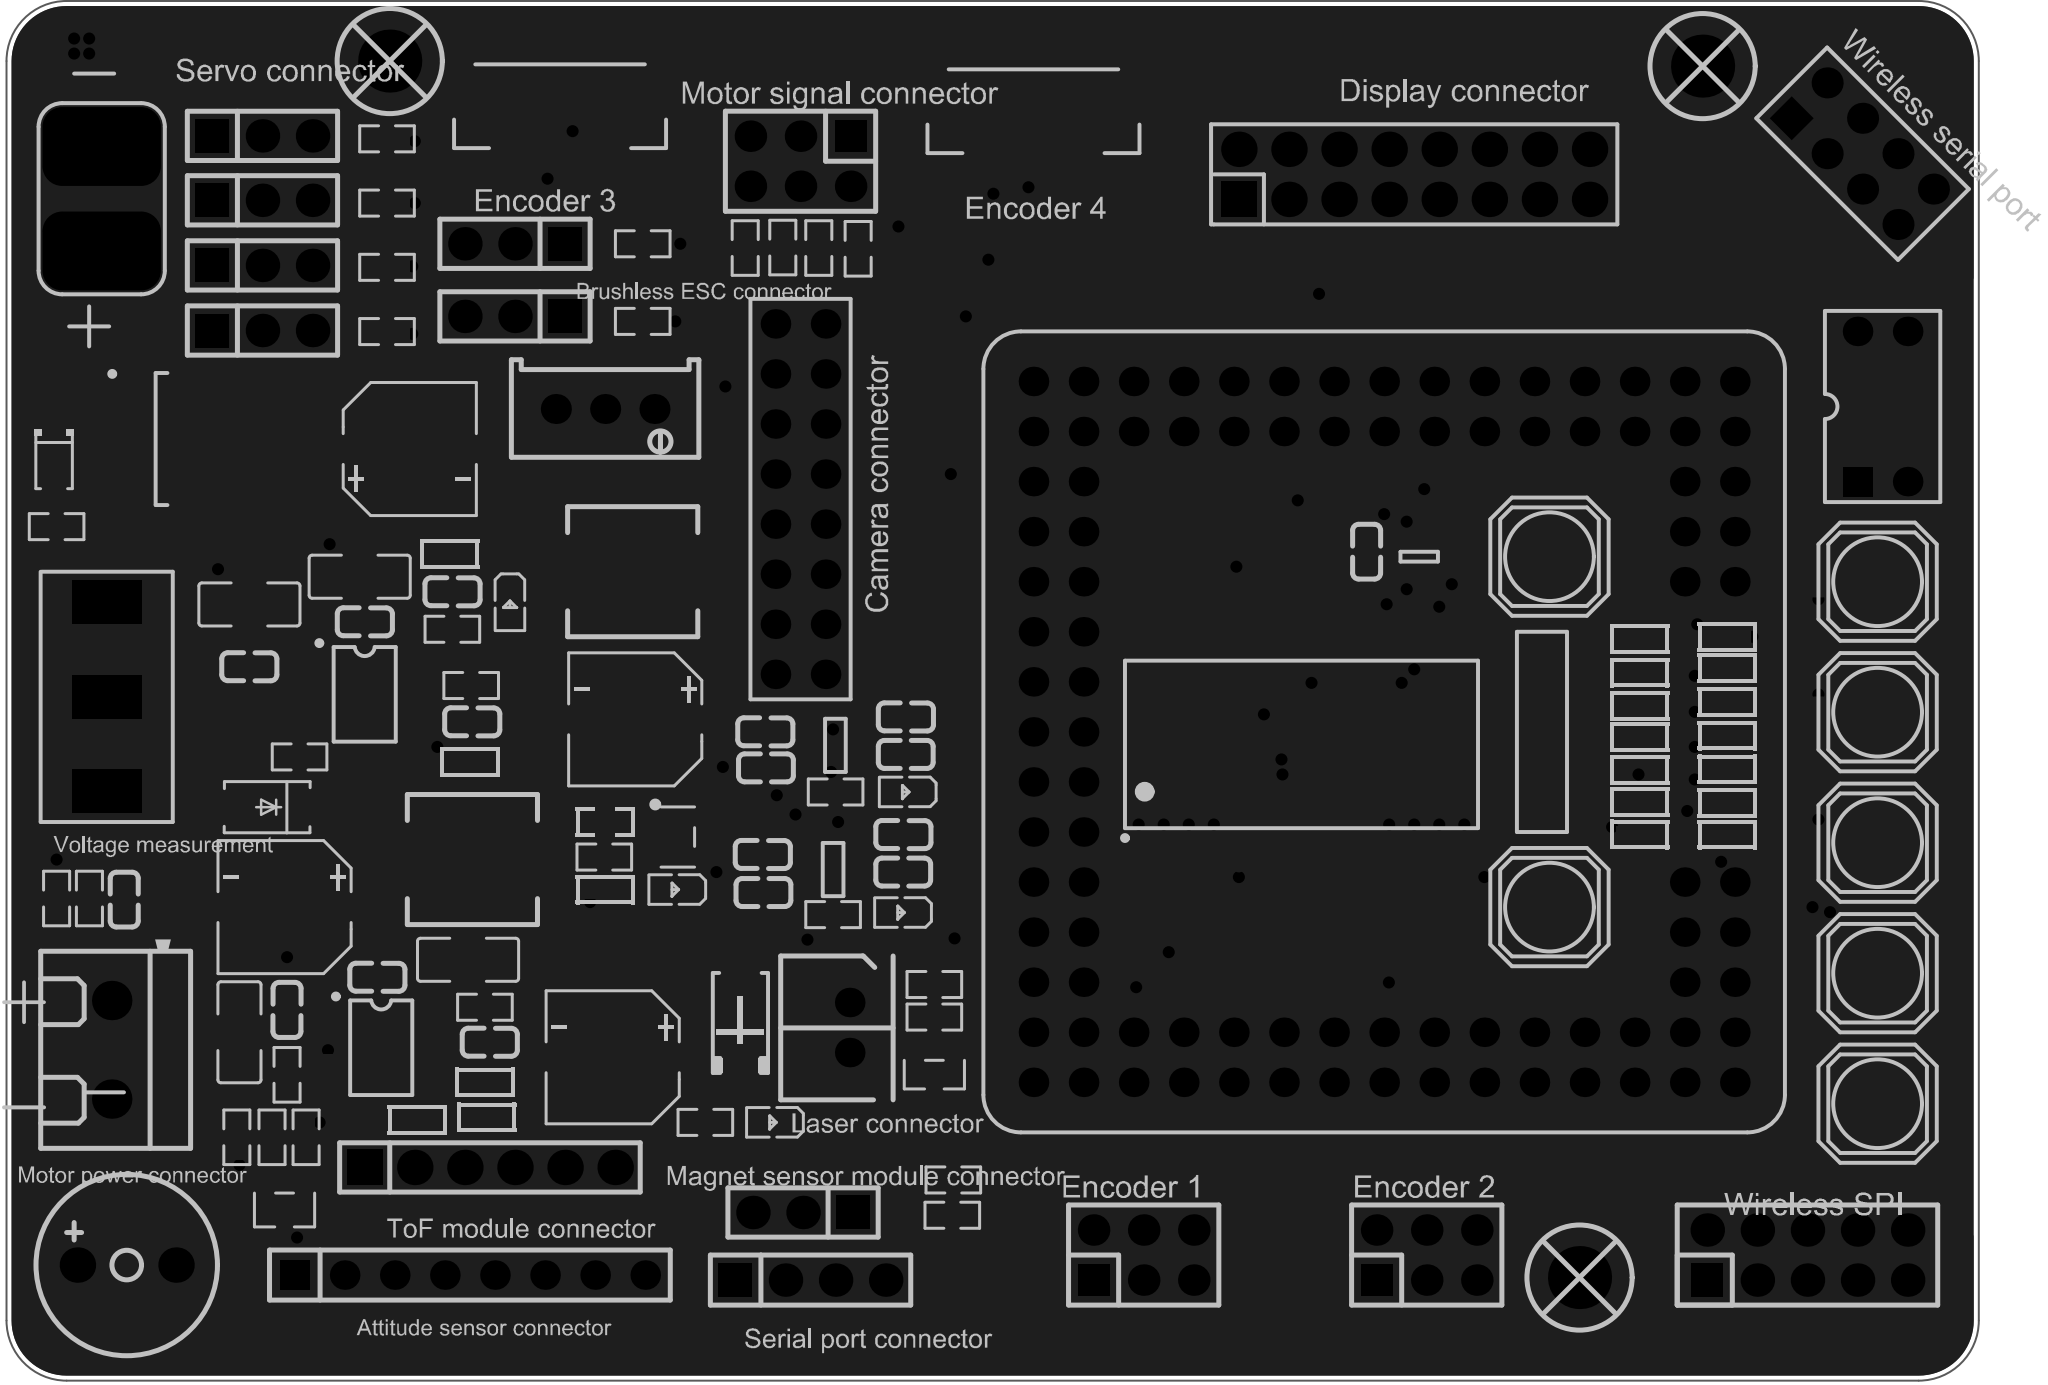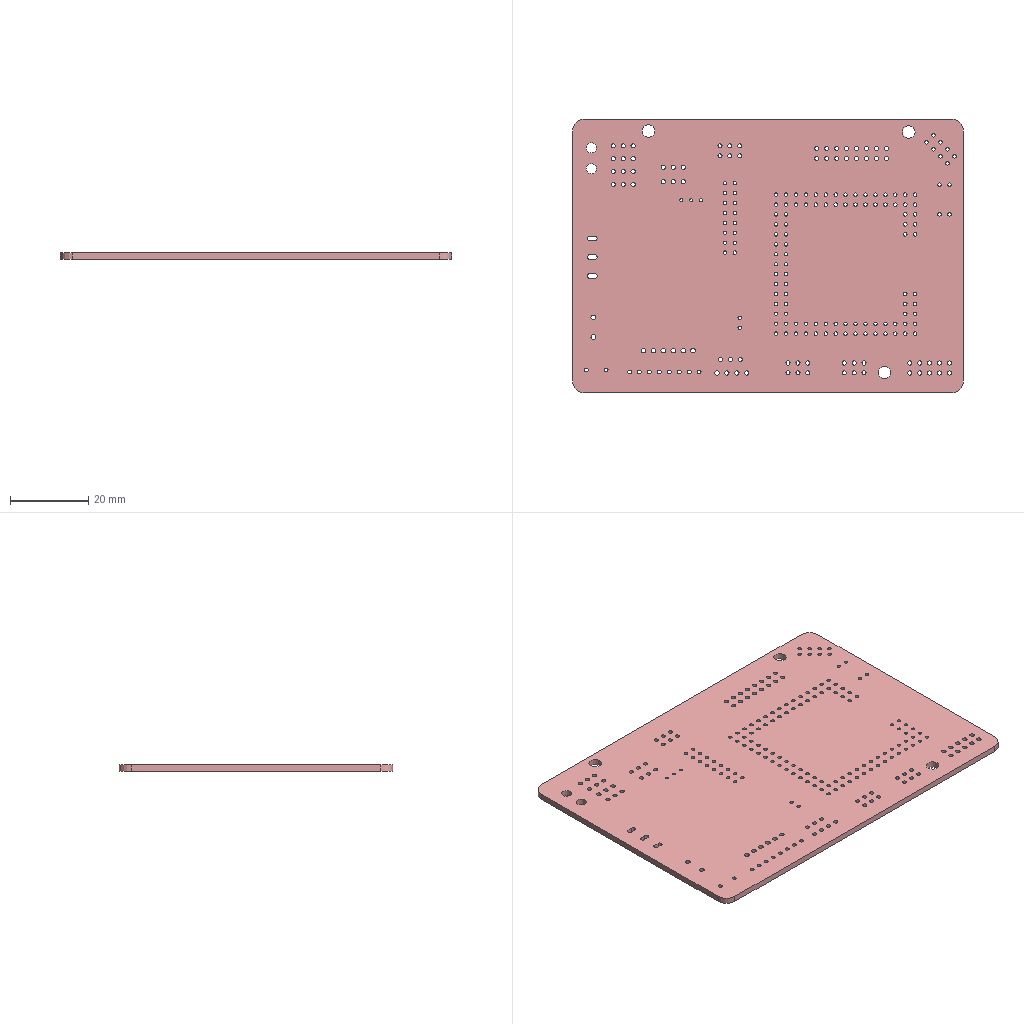Circuit board layout | Altium Designer | box 100 x 70 x 1.6 mm
Layer stack:
# Altium Designer layer stack of  (unit mm; dielectric type: 0 none, 1 core, 2 prepreg, 3 surface material)
index,name,kind,layer,copper_thickness_mm,dielectric_type,dielectric_thickness_mm,dielectric_material,dielectric_constant
0,Top Paste Mask Layer,other,,,,,,
1,Top Silkscreen Layer,other,,,,,,
2,Top Solder Mask Layer,dielectric,,,3,0,,0
3,Top Layer,copper,Top Layer,0.035,,,,
4,Dielectric1,dielectric,,,3,0.2104,7628 RC49% 8.6mil,0
5,Inner1,copper,Inner1,0.0152,,,,
6,Dielectric2,dielectric,,,3,1.065,1.1mm H/HOZ Copper,0
7,Inner2,copper,Inner2,0.0152,,,,
8,Dielectric3,dielectric,,,3,0.2104,7628 RC49% 8.6mil,0
9,Bottom Layer,copper,Bottom Layer,0.035,,,,
10,Bottom Solder Mask Layer,dielectric,,,3,0,,0
11,Bottom Silkscreen Layer,other,,,,,,
12,Bottom Paste Mask Layer,other,,,,,,
# drill layer pairs: low layer,high layer
drill_pair,Top Layer,Bottom Layer
Part placement:
Designator,Comment,Layer,Footprint,Center-X(mm),Center-Y(mm),Rotation
B1,3kHz,TopLayer,BUZ-TH_BD9.0-P5.00-D0.6-FD,86.867,86.995,0
C18,10uF,TopLayer,C0603,119.253,114.046,0
C29,100nF,TopLayer,CAPC1608[0603]S-N,111.125,109.474,180
C35,100uF,TopLayer,CAP-SMD_BD6.3-L6.6-W6.6-LS7.6-FD-1,101.219,128.397,0
C37,100nF,TopLayer,C0603,93.091,117.348,0
C38,100nF,TopLayer,C0603,98.933,119.634,180
C39,4.7nF,TopLayer,C0603,104.394,114.554,0
C43,10uF,TopLayer,C0603,126.365,114.808,180
C53,220uF,TopLayer,CAP-SMD_BD6.3-L6.6-W6.6-LS7.6-FD-1,112.649,114.681,180
C59,4.7uf,TopLayer,C1206,93.088,120.512,0
C60,47uf,TopLayer,C1206,98.679,121.92,0
C61,100uF,TopLayer,CAP-SMD_BD6.3-L6.6-W6.6-LS7.6-FD-1,94.869,105.156,180
C62,100nF,TopLayer,C0603,94.996,99.949,90
C63,100nF,TopLayer,C0603,99.568,101.6,180
C64,4.7nF,TopLayer,C0603,105.283,98.298,0
C65,220uF,TopLayer,CAP-SMD_BD6.3-L6.6-W6.6-LS7.6-FD-1,111.506,97.536,180
C66,4.7uf,TopLayer,C1206,92.583,98.806,90
C67,47uf,TopLayer,C1206,104.174,102.484,0
C68,100nF,TopLayer,C0603,103.378,121.158,180
C71,100nF,TopLayer,C0603,119.277,112.22,0
C72,100nF,TopLayer,C0603,126.365,112.903,180
C73,10uF,TopLayer,C0603,119.126,107.823,0
C74,10uF,TopLayer,C0603,126.238,108.839,180
C75,100nF,TopLayer,C0603,119.15,105.895,0
C76,100nF,TopLayer,C0603,126.238,106.934,180
C77,100nF,TopLayer,C0603,149.733,123.19,270
C78,100nF,TopLayer,C0603,86.741,105.537,90
D1,BZT52C16,TopLayer,SOD-123_L2.7-W1.6-LS3.7-RD,83.185,127.762,270
D6,SS54,TopLayer,SMA_L4.3-W2.6-LS5.0-FD,93.98,110.236,0
D7,SS54,TopLayer,SMA-L[DO-214AC],117.983,99.441,270
H1,,TopLayer,HDR-TH_16P-P2.54-V-F-R2-C8-S2.54-1,152.146,142.334,0
H2,,TopLayer,HDR-TH_10P-P2.54-V-F-R2-C5-S2.54,172.085,87.503,0
H3,,TopLayer,HDR-TH_4P-P2.54-V-M,121.539,86.233,0
H4,,TopLayer,HDR-TH_3P-P2.54-V-M,106.553,138.811,180
H6,,TopLayer,HDR-TH_3P-P2.54-V-M,106.553,135.128,180
H7,,TopLayer,HDR-TH_6P-P2.54-V-M-1,105.283,91.948,0
H8,,TopLayer,HDR-TH_8P-P2.54-V-M,104.267,86.487,0
H9,HDR-F-2.54_2x4,TopLayer,HDR-F-2.54_2X4,174.879,143.383,315
H11,,TopLayer,HDR-TH_6P-P2.54-V-R2-C3-S2.54_A2541WV-2X3P,138.43,87.503,0
H12,,TopLayer,HDR-TH_6P-P2.54-V-R2-C3-S2.54_A2541WV-2X3P,152.781,87.503,0
H15,,TopLayer,HDR-TH_3P-P2.54-V-M,121.158,89.662,180
H16,,TopLayer,HDR-TH_3P-P2.54-V-M,93.75,144.287,0
H17,,TopLayer,HDR-TH_3P-P2.54-V-M,93.75,141.017,0
H18,,TopLayer,HDR-TH_3P-P2.54-V-M,93.75,137.714,0
H19,,TopLayer,HDR-TH_3P-P2.54-V-M,93.75,134.411,0
H20,,TopLayer,HDR-TH_6P-P2.54-V-R2-C3-S2.54_A2541WV-2X3P,121.031,143,180
L3,4.7uH,TopLayer,IND-SMD_L7.2-W6.6_GPSR07X0,112.522,122.174,0
L4,4.7uH,TopLayer,IND-SMD_L7.2-W6.6_GPSR07X0,104.394,107.569,0
LED4,,TopLayer,LED_0603,106.291,120.574,270
LED5,,TopLayer,LED_0603,119.685,94.242,180
LED8,,TopLayer,LED_0603,114.732,106.053,180
LED9,,TopLayer,LED_0603,126.416,111.006,180
LED11,,TopLayer,LED_0603,126.178,104.887,180
P1,XT60_Header,TopLayer,Wired_T-Header_ThroughHole,85.598,141.097,180
P4,KF301-2P terminal block,TopLayer,CONN-TH_XY301V-A-5.0-2P,86.106,97.917,90
P5,GH1.25-6P-SH new encoder board end, horizontal,TopLayer,ECD-GH1.25-6P-SV,108.839,144.99,180
P6,GH1.25-6P-SH new encoder board end, horizontal,TopLayer,ECD-GH1.25-6P-SV,132.842,144.736,180
P7,XH2.54-2P,TopLayer,XH2.54-2P-DV,123.525,99.046,270
P8,Camera Interface,TopLayer,HDR2X8-F-High,121.031,125.857,270
Q1,HY19P03,TopLayer,TO-252AA,89.408,128.905,0
Q3,S8050,TopLayer,SOT-23-3_L3.0-W1.7-P0.95-LS2.9-BR,94.869,89.789,90
R1,10K,TopLayer,R0603,83.312,124.46,0
R18,2.7K,TopLayer,R0603,122.809,110.998,0
R21,10K,TopLayer,RESC1608[0603]S-N,111.125,106.045,0
R22,4.7K,TopLayer,R0603,111.082,107.696,0
R33,4.7K,TopLayer,R0603,95.962,93.477,270
R34,10K,TopLayer,R0603,94.234,93.477,270
R44,200K,TopLayer,R0603,95.631,112.776,0
R45,20K,TopLayer,R0603,104.332,116.399,0
R46,10K,TopLayer,R0603,103.378,119.253,0
R47,27K,TopLayer,RESC1608[0603]S-N,103.251,123.063,180
R49,8.2K,TopLayer,RESC1608[0603]S-N,104.267,112.522,180
R50,200K,TopLayer,R0603,94.996,96.647,270
R51,20K,TopLayer,R0603,105.029,100.076,0
R52,4.7K,TopLayer,R0603,116.205,94.234,0
R53,51K,TopLayer,RESC1608[0603]S-N,105.118,94.483,0
R54,1.5K,TopLayer,RESC1608[0603]S-N,105.029,96.266,0
R55,10K,TopLayer,RESC1608[0603]S-N,101.6,94.361,180
R56,50kΩ,TopLayer,RES-ADJ-TH_3P-L9.5-W4.85-P2.50-BL-BS,111.125,130.429,270
R58,2.7K,TopLayer,R0603,122.682,104.775,0
R59,100R,TopLayer,R0603,113.03,138.811,0
R60,100R,TopLayer,R0603,113.03,134.874,0
R61,100R,TopLayer,R0603,120.132,138.62,270
R62,100R,TopLayer,R0603,118.225,138.596,270
R63,100R,TopLayer,R0603,123.952,138.557,90
R64,10R,TopLayer,R0603,92.451,93.477,270
R74,4.7K,TopLayer,RESC1608[0603]S-N,168.021,118.872,180
R76,470R,TopLayer,RESC1608[0603]S-N,163.576,118.745,0
R77,100R,TopLayer,R0603,128.778,91.313,180
R78,10K,TopLayer,R0603,128.726,89.522,0
R79,100R,TopLayer,R0603,100.065,144.136,0
R80,100R,TopLayer,R0603,100.065,140.876,0
R81,100R,TopLayer,R0603,100.065,137.617,0
R82,100R,TopLayer,R0603,100.065,134.357,0
R83,100R,TopLayer,R0603,121.957,138.596,90
R84,100R,TopLayer,R0603,127.816,101.229,180
R85,10K,TopLayer,R0603,127.816,99.578,0
R86,470R,TopLayer,RESC1608[0603]S-N,163.576,117.052,0
R87,470R,TopLayer,RESC1608[0603]S-N,163.576,115.358,0
R88,470R,TopLayer,RESC1608[0603]S-N,163.576,113.792,0
R89,470R,TopLayer,RESC1608[0603]S-N,163.576,112.099,0
R91,4.7K,TopLayer,RESC1608[0603]S-N,168.021,113.856,180
R92,4.7K,TopLayer,RESC1608[0603]S-N,168.021,115.57,180
R93,4.7K,TopLayer,RESC1608[0603]S-N,168.021,117.284,180
R94,4.7K,TopLayer,RESC1608[0603]S-N,168.021,112.141,180
R95,4.7K,TopLayer,RESC1608[0603]S-N,168.021,108.839,180
R96,4.7K,TopLayer,RESC1608[0603]S-N,168.021,110.427,180
R97,470R,TopLayer,RESC1608[0603]S-N,163.576,110.49,0
R98,470R,TopLayer,RESC1608[0603]S-N,163.576,108.839,0
R99,20K,TopLayer,R0603,84.976,105.593,90
R100,200K,TopLayer,R0603,83.312,105.593,270
S2,SW DIP-2,TopLayer,Code_SW-2-DIP-2.54,175.895,130.555,0
S3,KEY-TS1145,TopLayer,TS-1199A,175.641,95.182,180
S4,KEY-TS1145,TopLayer,TS-1199A,175.641,101.803,180
S5,KEY-TS1145,TopLayer,TS-1199A,175.641,108.424,180
S6,KEY-TS1145,TopLayer,TS-1199A,175.641,115.045,180
S7,KEY-TS1145,TopLayer,TS-1199A,175.641,121.666,180
SCREW1,,TopLayer,M3螺丝,166.768,147.826,0
SCREW2,,TopLayer,M3螺丝,100.203,148.082,0
SCREW3,,TopLayer,M3螺丝,160.528,86.36,0
U1,STC32G144K246_CoreBoard,TopLayer,STC32G144K246_CoreBoard,150.622,114.046,0
U2,,TopLayer,SS12D10,85.852,115.824,270
U4,RT9013-33,TopLayer,SOT-23-5,122.799,113.363,0
U7,SY6280,TopLayer,SOT-23-5_L3.0-W1.7-P0.95-LS2.8-BL,114.808,108.712,270
U13,SCT2450,TopLayer,SOP-8E,98.933,115.951,0
U14,SCT2450,TopLayer,SOP-8E,99.771,98.021,0
U16,RT9013-33,TopLayer,SOT-23-5,122.682,107.061,0
U17,AL422B,TopLayer,SOP-28,146.431,113.411,90
U18,SN74LVC1G00DCKR,TopLayer,SOT-353,152.4,122.936,90
U19,AO3400,TopLayer,SOT-23-3_L2.9-W1.3-P1.90-LS2.4-BL-2,127.816,96.657,180
Pad and via stacks:
# Altium Designer via and pad stacks of  (unit mm). Each distinct definition once, with the count of objects using it.
# via: kind,start_layer,end_layer,hole_mm,diameter_mm,mode(0 simple;1 top-mid-bottom;2 full stack),diameter_per_layer,count,example_net
# pad: kind,layer,hole_mm,hole_type(0 round;1 square;2 slot),plating,top_size,top_shape(1 round;2 rect;3 octagon;9 rounded rect),mid_size,bottom_size,mode,footprint,size_per_layer,count,example
pad,Multi-Layer,1,0,plated,1.8x1.8,1,1.8x1.8,1.8x1.8,0,BUZ-TH_BD9.0-P5.00-D0.6-FD,,2,B1.1
pad,Multi-Layer,1.1,0,plated,1.8x1.8,1,1.8x1.8,1.8x1.8,0,HDR-TH_16P-P2.54-V-F-R2-C8-S2.54-1,,15,H1.16
pad,Multi-Layer,1.1,0,plated,1.8x1.8,2,1.8x1.8,1.8x1.8,0,HDR-TH_16P-P2.54-V-F-R2-C8-S2.54-1,,1,H1.1
pad,Multi-Layer,1.1,0,plated,1.7x1.7,1,1.7x1.7,1.7x1.7,0,HDR-TH_10P-P2.54-V-F-R2-C5-S2.54,,9,H2.10
pad,Multi-Layer,1.1,0,plated,1.575x1.7,2,1.575x1.7,1.575x1.7,0,HDR-TH_10P-P2.54-V-F-R2-C5-S2.54,,1,H2.1
pad,Multi-Layer,1.1,0,plated,1.7x1.7,2,1.7x1.7,1.7x1.7,0,HDR-TH_4P-P2.54-V-M,,1,H3.1
pad,Multi-Layer,1.1,0,plated,1.7x1.7,1,1.7x1.7,1.7x1.7,0,HDR-TH_4P-P2.54-V-M,,3,H3.2
pad,Multi-Layer,1.1,0,plated,1.7x1.7,2,1.7x1.7,1.7x1.7,0,HDR-TH_3P-P2.54-V-M,,7,H4.1
pad,Multi-Layer,1.1,0,plated,1.7x1.7,1,1.7x1.7,1.7x1.7,0,HDR-TH_3P-P2.54-V-M,,14,H4.2
pad,Multi-Layer,1.2,0,plated,1.8x1.8,1,1.8x1.8,1.8x1.8,0,HDR-TH_6P-P2.54-V-M-1,,5,H7.6
pad,Multi-Layer,1.2,0,plated,1.8x1.8,2,1.8x1.8,1.8x1.8,0,HDR-TH_6P-P2.54-V-M-1,,1,H7.1
pad,Multi-Layer,1,0,plated,1.5x1.5,2,1.5x1.5,1.5x1.5,0,HDR-TH_8P-P2.54-V-M,,1,H8.1
pad,Multi-Layer,1,0,plated,1.5x1.5,1,1.5x1.5,1.5x1.5,0,HDR-TH_8P-P2.54-V-M,,7,H8.2
pad,Multi-Layer,0.889,0,plated,1.575x1.575,2,1.575x1.575,1.575x1.575,0,HDR-F-2.54_2X4,,1,H9.1
pad,Multi-Layer,0.889,0,plated,1.575x1.575,1,1.575x1.575,1.575x1.575,0,HDR-F-2.54_2X4,,7,H9.2
pad,Multi-Layer,1.05,0,plated,1.6x1.6,2,1.6x1.6,1.6x1.6,0,HDR-TH_6P-P2.54-V-R2-C3-S2.54_A2541WV-2X3P,,3,H11.1
pad,Multi-Layer,1.05,0,plated,1.6x1.6,1,1.6x1.6,1.6x1.6,0,HDR-TH_6P-P2.54-V-R2-C3-S2.54_A2541WV-2X3P,,15,H11.2
pad,Multi-Layer,2.6,0,plated,6x4,9,6x4,6x4,0,Wired T-Header ThroughHole,,2,P1.1
pad,Multi-Layer,1.2,0,plated,2x2,1,2x2,2x2,0,CONN-TH_XY301V-A-5.0-2P,,2,P4.1
pad,Multi-Layer,0.9,0,plated,1.5x1.5,1,1.5x1.5,1.5x1.5,0,XH2.54-2P-DV,,2,P7.1
pad,Multi-Layer,0.9,0,plated,1.5x1.5,1,1.5x1.5,1.5x1.5,0,HDR2X8-F-High,,16,P8.15
pad,Multi-Layer,0.762,0,plated,1.524x1.524,1,1.524x1.524,1.524x1.524,0,RES-ADJ-TH_3P-L9.5-W4.85-P2.50-BL-BS,,3,R56.2
pad,Multi-Layer,0.9,0,plated,1.5x1.5,1,1.5x1.5,1.5x1.5,0,Code SW-2-DIP-2.54,,3,S2.3
pad,Multi-Layer,0.9,0,plated,1.5x1.5,2,1.5x1.5,1.5x1.5,0,Code SW-2-DIP-2.54,,1,S2.1
pad,Multi-Layer,3.2,0,plated,3.2x3.2,1,3.2x3.2,3.2x3.2,0,M3\u00C2\u00DD\u00CB\u00BF,,3,SCREW1.1
pad,Multi-Layer,0.9,0,plated,1.5x1.5,1,1.5x1.5,1.5x1.5,0,STC32G144K246_CoreBoard,,94,U1.6
pad,Multi-Layer,1.2,2,plated,2.2x3.5,2,2.2x3.5,2.2x3.5,0,SS12D10,,3,U2.3
pad,Top Layer,0,0,plated,0.8x0.9,2,0.8x0.9,0.8x0.9,0,C0603,,34,C18.2
pad,Top Layer,0,0,plated,0.9x0.8,2,0.9x0.8,0.9x0.8,0,CAPC1608[0603]S-N,,2,C29.1
pad,Top Layer,0,0,plated,3.5x1.2,2,3.5x1.2,3.5x1.2,0,CAP-SMD_BD6.3-L6.6-W6.6-LS7.6-FD-1,,8,C35.1
pad,Top Layer,0,0,plated,1.485x1.728,2,1.485x1.728,1.485x1.728,0,C1206,,8,C59.2
pad,Top Layer,0,0,plated,0.91x1.22,2,0.91x1.22,0.91x1.22,0,SOD-123_L2.7-W1.6-LS3.7-RD,,2,D1.2
pad,Top Layer,0,0,plated,2.046x1.62,2,2.046x1.62,2.046x1.62,0,SMA_L4.3-W2.6-LS5.0-FD,,2,D6.1
pad,Top Layer,0,0,plated,2x1.75,2,2x1.75,2x1.75,0,SMA-L[DO-214AC],,2,D7.A
pad,Top Layer,0,0,plated,2.35x3.5,2,2.35x3.5,2.35x3.5,0,IND-SMD_L7.2-W6.6_GPSR07X0,,4,L3.1
pad,Top Layer,0,0,plated,0.8001x0.8001,2,0.8001x0.8001,0.8001x0.8001,0,LED_0603,,10,LED4.1
pad,Top Layer,0,0,plated,1x2.8,2,1x2.8,1x2.8,0,ECD-GH1.25-6P-SV,,4,P5.0
pad,Top Layer,0,0,plated,0.6x1.7,2,0.6x1.7,0.6x1.7,0,ECD-GH1.25-6P-SV,,12,P5.6
pad,Top Layer,0,0,plated,5.5x6.7,2,5.5x6.7,5.5x6.7,0,TO-252AA,,1,Q1.1
pad,Top Layer,0,0,plated,0.95x2.2,2,0.95x2.2,0.95x2.2,0,TO-252AA,,2,Q1.3
pad,Top Layer,0,0,plated,1.038x0.532,2,1.038x0.532,1.038x0.532,0,SOT-23-3_L3.0-W1.7-P0.95-LS2.9-BR,,3,Q3.1
pad,Top Layer,0,0,plated,0.8065x0.864,2,0.8065x0.864,0.8065x0.864,0,R0603,,58,R1.2
pad,Top Layer,0,0,plated,0.9x0.8,2,0.9x0.8,0.9x0.8,0,RESC1608[0603]S-N,,40,R21.2
pad,Top Layer,0,0,plated,2x1.6,1,2x1.6,2x1.6,0,TS-1199A,,10,S3.2
pad,Top Layer,0,0,plated,0.6x1.1,2,0.6x1.1,0.6x1.1,0,SOT-23-5,,10,U4.3
pad,Top Layer,0,0,plated,0.49x1.157,2,0.49x1.157,0.49x1.157,0,SOT-23-5_L3.0-W1.7-P0.95-LS2.8-BL,,3,U7.1
pad,Top Layer,0,0,plated,0.49x1.175,2,0.49x1.175,0.49x1.175,0,SOT-23-5_L3.0-W1.7-P0.95-LS2.8-BL,,2,U7.4
pad,Top Layer,0,0,unplated,2.5x3.4,2,2.5x3.4,2.5x3.4,0,SOP-8E,,2,U13.9
pad,Top Layer,0,0,unplated,1.6x0.65,2,1.6x0.65,1.6x0.65,0,SOP-8E,,16,U13.1
pad,Top Layer,0,0,unplated,2x0.6,1,2x0.6,2x0.6,0,SOP-28,,28,U17.5
pad,Top Layer,0,0,plated,0.4x0.8,2,0.4x0.8,0.4x0.8,0,SOT-353,,5,U18.4
pad,Top Layer,0,0,plated,1.25x0.7,2,1.25x0.7,1.25x0.7,0,SOT-23-3_L2.9-W1.3-P1.90-LS2.4-BL-2,,3,U19.3
via,Top Layer,Bottom Layer,0.3048,0.61,0,,82,2.4
Copper pours:
name,layer,net,type(0 solid;1 hatched;2 none)
Top Layer-GND,Top Layer,GND,0
Bottom Layer-GND,Bottom Layer,GND,0
Design rules, without the lines most boards share:
# Altium Designer design rules of  (exported by Altium Designer, unit mm)
# columns: name | kind | enabled | priority | scope1 | scope2 | descriptor | typed fields (field=value)
copperRegion | 20 | enabled | 1 | All | All | Polygon Connect Rule(Direct Connect )(Conductor Width=10mil) (Relief Angle=90 Angle) (Entries=4) (Air Gap Width=10mil) (All),(All) | connect_style(0=relief,1=direct,2=none)=1 relief_conductor_width=0.254 relief_entries=4